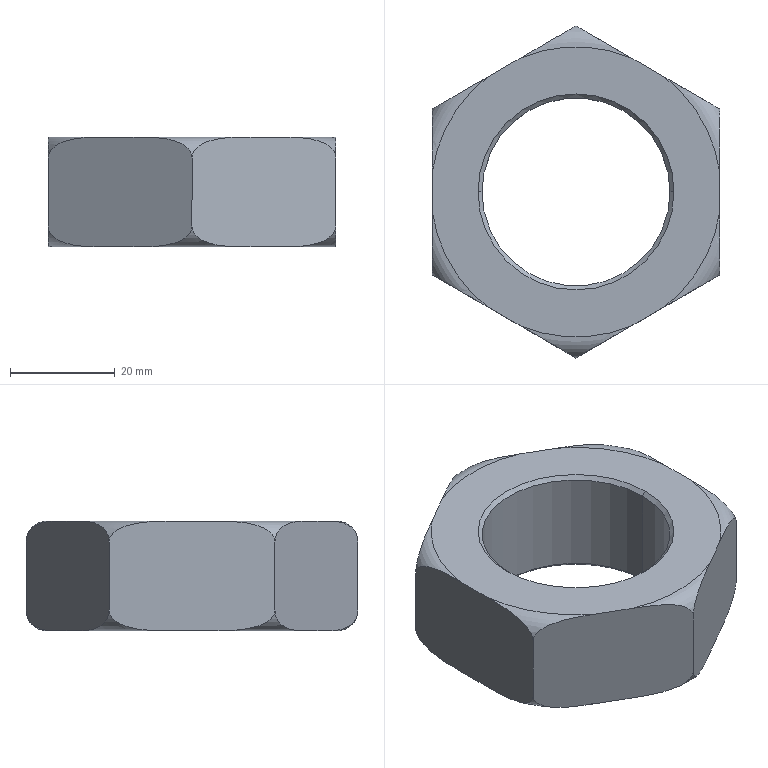Part | STEP file | NT-16_CS1-RodEndNut | 1 solid | 26 faces | box 55 x 63.509 x 21 mm | volume 33434 mm3 | torus 12 | plane 8 | cone 4 | cylinder 2 | commonest cylinder face diameters 36 x2